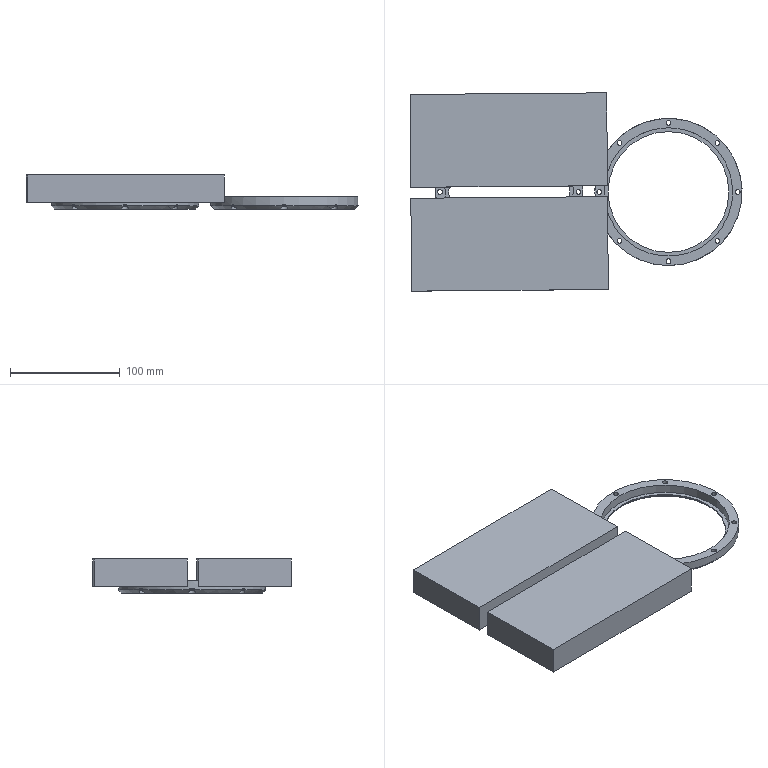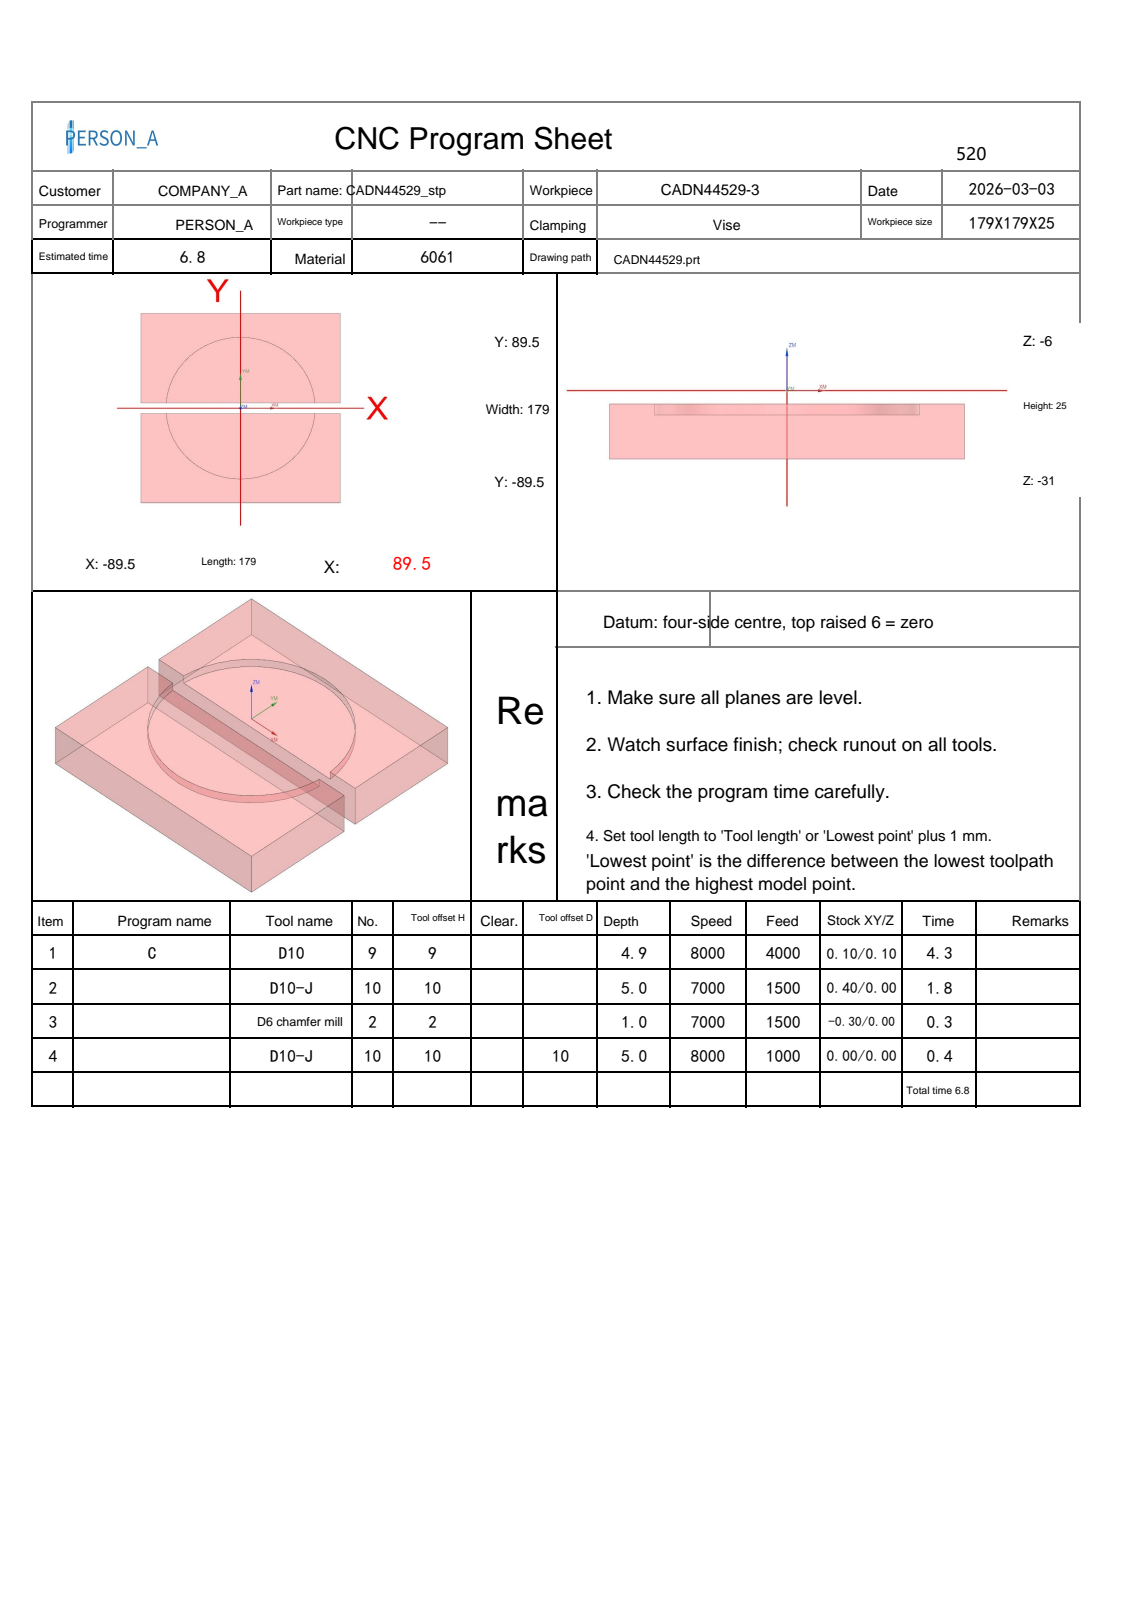NC program | NX | posted by the shop | part box 302.234 x 180.468 x 31 mm
Whole program:
%
O0001
(Machine time: 7.55 MIN)
(===Total Tool:3===)
(T9=D10     D=10.  R=0.   D-  H09 Z=-10.9 )
(T10=D10-J  D=10.  R=0.   D-  H10 Z=-11.  )
(T2=D6 chamfer mill   D=6.   R=0.   D-  H02 Z=-7.   )
G80 G90 G17 G49 G40
G91 G28 Z0
M01
N1 T09 M06
(D10  D=10. R=0. H=09 ce=0.10 di=0.10)
G00 G90 G54 X5.978 Y2.842 M03 S8000
G43 H09 Z4.1
M08
Z-4.5
G03 X5.978 Y2.842 Z-5.982 I-3.383 J-2.967 F4000.
X-1.902 Y.036 Z-6.544 I-3.383 J-2.967
G01 X-1.9 Y-.07
G03 X-.001 Y-1.9 I1.899 J.07
G01 X.142 Y-1.895
G03 X1.895 Y-.142 I-.142 J1.895
G01 X1.9 Y-.07
Y.07
G03 X.001 Y1.9 I-1.899 J-.07
G01 X-.142 Y1.895
X-.304 Y1.876
G03 X-.536 Y1.808 I.16 J-.987
G01 X-8.42 Y-1.553
G03 X-9.028 Y-2.473 I.392 J-.92
X-8.984 Y-2.767 I1. J0.0
X0.0 Y-9.4 I8.984 J2.767
X9.374 Y-.701 I0.0 J9.4
G01 X9.421 Y-.07
Y.07
X9.374 Y.701
G03 X0.0 Y9.4 I-9.374 J-.701
X-8.773 Y3.376 I0.0 J-9.4
G02 X-9.224 Y2.859 I-.933 J.359
G01 X-16.269 Y-1.02
G03 X-16.787 Y-1.896 I.483 J-.876
G01 X-16.779 Y-2.015
G03 X0.0 Y-16.9 I16.779 J2.015
X16.853 Y-1.261 I0.0 J16.9
G01 X16.942 Y-.071
Y.071
X16.853 Y1.261
G03 X0.0 Y16.9 I-16.853 J-1.261
X-16.409 Y4.046 I0.0 J-16.9
G02 X-16.892 Y3.412 I-.971 J.24
G01 X-23.852 Y-.467
G03 X-24.365 Y-1.341 I.487 J-.873
G01 X-24.362 Y-1.415
X-24.332 Y-1.821
G03 X0.0 Y-24.4 I24.332 J1.821
X24.332 Y-1.821 I0.0 J24.4
G01 X24.463 Y-.071
Y.071
X24.332 Y1.821
G03 X0.0 Y24.4 I-24.332 J-1.821
X-23.953 Y4.649 I0.0 J-24.4
G02 X-24.448 Y3.967 I-.982 J.191
G01 X-31.414 Y.092
G03 X-31.928 Y-.782 I.486 J-.874
G01 X-31.925 Y-.856
X-31.811 Y-2.381
G03 X0.0 Y-31.9 I31.811 J2.381
X31.811 Y-2.381 I0.0 J31.9
G01 X31.984 Y-.071
Y.071
X31.811 Y2.381
G03 X0.0 Y31.9 I-31.811 J-2.381
X-31.468 Y5.232 I0.0 J-31.9
G02 X-31.968 Y4.522 I-.986 J.164
G01 X-38.975 Y.625
G03 X-39.489 Y-.249 I.487 J-.874
G01 X-39.486 Y-.323
X-39.29 Y-2.94
G03 X0.0 Y-39.4 I39.29 J2.94
X39.29 Y-2.94 I0.0 J39.4
G01 X39.505 Y-.071
Y.071
X39.29 Y2.94
G03 X0.0 Y39.4 I-39.29 J-2.94
X-38.97 Y5.805 I0.0 J-39.4
G02 X-39.472 Y5.079 I-.989 J.148
G01 X-46.494 Y1.163
G03 X-47.004 Y.365 I.488 J-.873
G01 X-47.026 Y.072
Y-.072
X-46.769 Y-3.5
G03 X0.0 Y-46.9 I46.769 J3.5
X46.769 Y-3.5 I0.0 J46.9
G01 X47.026 Y-.072
Y.072
X46.769 Y3.5
G03 X0.0 Y46.9 I-46.769 J-3.5
X-46.465 Y6.373 I0.0 J-46.9
G02 X-46.967 Y5.637 I-.991 J.136
G01 X-53.974 Y1.723
G03 X-54.483 Y.925 I.488 J-.873
G01 X-54.547 Y.072
Y-.072
X-54.248 Y-4.06
G03 X0.0 Y-54.4 I54.248 J4.06
X54.248 Y-4.06 I0.0 J54.4
G01 X54.547 Y-.072
Y.072
X54.248 Y4.06
G03 X0.0 Y54.4 I-54.248 J-4.06
X-53.923 Y7.188 I0.0 J-54.4
G02 X-54.768 Y6.331 I-.991 J.133
G01 X-60.884 Y5.428
G03 X-61.735 Y4.513 I.146 J-.989
G01 X-62.073 Y0.0
X-61.727 Y-4.619
G03 X0.0 Y-61.9 I61.727 J4.619
X61.727 Y-4.619 I0.0 J61.9
G01 X62.073 Y0.0
X61.727 Y4.619
G03 X0.0 Y61.9 I-61.727 J-4.619
X-61.727 Y4.619 I0.0 J-61.9
G01 X-62.073 Y0.0
X-62.038 Y-.473
X-62. Y-.971
X-59.009 Y-.747
Z-5.044
G00 X5.978 Y2.842
G03 X5.978 Y2.842 Z-6.526 I-3.383 J-2.967
X-1.902 Y.036 Z-7.089 I-3.383 J-2.967
G01 X-1.9 Y-.07
G03 X-.001 Y-1.9 I1.899 J.07
G01 X.142 Y-1.895
G03 X1.895 Y-.142 I-.142 J1.895
G01 X1.9 Y-.07
Y.07
G03 X.001 Y1.9 I-1.899 J-.07
G01 X-.142 Y1.895
X-.304 Y1.876
G03 X-.536 Y1.808 I.16 J-.987
G01 X-8.42 Y-1.553
G03 X-9.028 Y-2.473 I.392 J-.92
X-8.984 Y-2.767 I1. J0.0
X0.0 Y-9.4 I8.984 J2.767
X9.374 Y-.701 I0.0 J9.4
G01 X9.421 Y-.07
Y.07
X9.374 Y.701
G03 X0.0 Y9.4 I-9.374 J-.701
X-8.773 Y3.376 I0.0 J-9.4
G02 X-9.224 Y2.859 I-.933 J.359
G01 X-16.269 Y-1.02
G03 X-16.787 Y-1.896 I.483 J-.876
G01 X-16.779 Y-2.015
G03 X0.0 Y-16.9 I16.779 J2.015
X16.853 Y-1.261 I0.0 J16.9
G01 X16.942 Y-.071
Y.071
X16.853 Y1.261
G03 X0.0 Y16.9 I-16.853 J-1.261
X-16.409 Y4.046 I0.0 J-16.9
G02 X-16.892 Y3.412 I-.971 J.24
G01 X-23.852 Y-.467
G03 X-24.365 Y-1.341 I.487 J-.873
G01 X-24.362 Y-1.415
X-24.332 Y-1.821
G03 X0.0 Y-24.4 I24.332 J1.821
X24.332 Y-1.821 I0.0 J24.4
G01 X24.463 Y-.071
Y.071
X24.332 Y1.821
G03 X0.0 Y24.4 I-24.332 J-1.821
X-23.953 Y4.649 I0.0 J-24.4
G02 X-24.448 Y3.967 I-.982 J.191
G01 X-31.414 Y.092
G03 X-31.928 Y-.782 I.486 J-.874
G01 X-31.925 Y-.856
X-31.811 Y-2.381
G03 X0.0 Y-31.9 I31.811 J2.381
X31.811 Y-2.381 I0.0 J31.9
G01 X31.984 Y-.071
Y.071
X31.811 Y2.381
G03 X0.0 Y31.9 I-31.811 J-2.381
X-31.468 Y5.232 I0.0 J-31.9
G02 X-31.968 Y4.522 I-.986 J.164
G01 X-38.975 Y.625
G03 X-39.489 Y-.249 I.487 J-.874
G01 X-39.486 Y-.323
X-39.29 Y-2.94
G03 X0.0 Y-39.4 I39.29 J2.94
X39.29 Y-2.94 I0.0 J39.4
G01 X39.505 Y-.071
Y.071
X39.29 Y2.94
G03 X0.0 Y39.4 I-39.29 J-2.94
X-38.97 Y5.805 I0.0 J-39.4
G02 X-39.472 Y5.079 I-.989 J.148
G01 X-46.494 Y1.163
G03 X-47.004 Y.365 I.488 J-.873
G01 X-47.026 Y.072
Y-.072
X-46.769 Y-3.5
G03 X0.0 Y-46.9 I46.769 J3.5
X46.769 Y-3.5 I0.0 J46.9
G01 X47.026 Y-.072
Y.072
X46.769 Y3.5
G03 X0.0 Y46.9 I-46.769 J-3.5
X-46.465 Y6.373 I0.0 J-46.9
G02 X-46.967 Y5.637 I-.991 J.136
G01 X-53.974 Y1.723
G03 X-54.483 Y.925 I.488 J-.873
G01 X-54.547 Y.072
Y-.072
X-54.248 Y-4.06
G03 X0.0 Y-54.4 I54.248 J4.06
X54.248 Y-4.06 I0.0 J54.4
G01 X54.547 Y-.072
Y.072
X54.248 Y4.06
G03 X0.0 Y54.4 I-54.248 J-4.06
X-53.923 Y7.188 I0.0 J-54.4
G02 X-54.768 Y6.331 I-.991 J.133
G01 X-60.884 Y5.428
G03 X-61.735 Y4.513 I.146 J-.989
G01 X-62.073 Y0.0
X-61.727 Y-4.619
G03 X0.0 Y-61.9 I61.727 J4.619
X61.727 Y-4.619 I0.0 J61.9
G01 X62.073 Y0.0
X61.727 Y4.619
G03 X0.0 Y61.9 I-61.727 J-4.619
X-61.727 Y4.619 I0.0 J-61.9
G01 X-62.073 Y0.0
X-62.038 Y-.473
X-62. Y-.971
X-59.009 Y-.747
Z-5.589
G00 X5.978 Y2.842
G03 X5.978 Y2.842 Z-7.071 I-3.383 J-2.967
X-1.902 Y.036 Z-7.633 I-3.383 J-2.967
G01 X-1.9 Y-.07
G03 X-.001 Y-1.9 I1.899 J.07
G01 X.142 Y-1.895
G03 X1.895 Y-.142 I-.142 J1.895
G01 X1.9 Y-.07
Y.07
G03 X.001 Y1.9 I-1.899 J-.07
G01 X-.142 Y1.895
X-.304 Y1.876
G03 X-.536 Y1.808 I.16 J-.987
G01 X-8.42 Y-1.553
G03 X-9.028 Y-2.473 I.392 J-.92
X-8.984 Y-2.767 I1. J0.0
X0.0 Y-9.4 I8.984 J2.767
X9.374 Y-.701 I0.0 J9.4
G01 X9.421 Y-.07
Y.07
X9.374 Y.701
G03 X0.0 Y9.4 I-9.374 J-.701
X-8.773 Y3.376 I0.0 J-9.4
G02 X-9.224 Y2.859 I-.933 J.359
G01 X-16.269 Y-1.02
G03 X-16.787 Y-1.896 I.483 J-.876
G01 X-16.779 Y-2.015
G03 X0.0 Y-16.9 I16.779 J2.015
X16.853 Y-1.261 I0.0 J16.9
G01 X16.942 Y-.071
Y.071
X16.853 Y1.261
G03 X0.0 Y16.9 I-16.853 J-1.261
X-16.409 Y4.046 I0.0 J-16.9
G02 X-16.892 Y3.412 I-.971 J.24
G01 X-23.852 Y-.467
G03 X-24.365 Y-1.341 I.487 J-.873
G01 X-24.362 Y-1.415
X-24.332 Y-1.821
G03 X0.0 Y-24.4 I24.332 J1.821
X24.332 Y-1.821 I0.0 J24.4
G01 X24.463 Y-.071
Y.071
X24.332 Y1.821
G03 X0.0 Y24.4 I-24.332 J-1.821
X-23.953 Y4.649 I0.0 J-24.4
G02 X-24.448 Y3.967 I-.982 J.191
G01 X-31.414 Y.092
G03 X-31.928 Y-.782 I.486 J-.874
G01 X-31.925 Y-.856
X-31.811 Y-2.381
G03 X0.0 Y-31.9 I31.811 J2.381
X31.811 Y-2.381 I0.0 J31.9
G01 X31.984 Y-.071
Y.071
X31.811 Y2.381
G03 X0.0 Y31.9 I-31.811 J-2.381
X-31.468 Y5.232 I0.0 J-31.9
G02 X-31.968 Y4.522 I-.986 J.164
G01 X-38.975 Y.625
G03 X-39.489 Y-.249 I.487 J-.874
G01 X-39.486 Y-.323
X-39.29 Y-2.94
G03 X0.0 Y-39.4 I39.29 J2.94
X39.29 Y-2.94 I0.0 J39.4
G01 X39.505 Y-.071
Y.071
X39.29 Y2.94
G03 X0.0 Y39.4 I-39.29 J-2.94
X-38.97 Y5.805 I0.0 J-39.4
G02 X-39.472 Y5.079 I-.989 J.148
G01 X-46.494 Y1.163
G03 X-47.004 Y.365 I.488 J-.873
G01 X-47.026 Y.072
Y-.072
X-46.769 Y-3.5
G03 X0.0 Y-46.9 I46.769 J3.5
X46.769 Y-3.5 I0.0 J46.9
G01 X47.026 Y-.072
Y.072
X46.769 Y3.5
G03 X0.0 Y46.9 I-46.769 J-3.5
X-46.465 Y6.373 I0.0 J-46.9
G02 X-46.967 Y5.637 I-.991 J.136
G01 X-53.974 Y1.723
G03 X-54.483 Y.925 I.488 J-.873
G01 X-54.547 Y.072
Y-.072
X-54.248 Y-4.06
G03 X0.0 Y-54.4 I54.248 J4.06
X54.248 Y-4.06 I0.0 J54.4
G01 X54.547 Y-.072
Y.072
X54.248 Y4.06
G03 X0.0 Y54.4 I-54.248 J-4.06
X-53.923 Y7.188 I0.0 J-54.4
G02 X-54.768 Y6.331 I-.991 J.133
G01 X-60.884 Y5.428
G03 X-61.735 Y4.513 I.146 J-.989
G01 X-62.073 Y0.0
X-61.727 Y-4.619
G03 X0.0 Y-61.9 I61.727 J4.619
X61.727 Y-4.619 I0.0 J61.9
G01 X62.073 Y0.0
X61.727 Y4.619
G03 X0.0 Y61.9 I-61.727 J-4.619
X-61.727 Y4.619 I0.0 J-61.9
G01 X-62.073 Y0.0
X-62.038 Y-.473
X-62. Y-.971
X-59.009 Y-.747
Z-6.133
G00 X5.978 Y2.842
G03 X5.978 Y2.842 Z-7.615 I-3.383 J-2.967
X-1.902 Y.036 Z-8.178 I-3.383 J-2.967
G01 X-1.9 Y-.07
G03 X-.001 Y-1.9 I1.899 J.07
G01 X.142 Y-1.895
G03 X1.895 Y-.142 I-.142 J1.895
G01 X1.9 Y-.07
Y.07
G03 X.001 Y1.9 I-1.899 J-.07
G01 X-.142 Y1.895
X-.304 Y1.876
G03 X-.536 Y1.808 I.16 J-.987
G01 X-8.42 Y-1.553
G03 X-9.028 Y-2.473 I.392 J-.92
X-8.984 Y-2.767 I1. J0.0
X0.0 Y-9.4 I8.984 J2.767
X9.374 Y-.701 I0.0 J9.4
G01 X9.421 Y-.07
Y.07
X9.374 Y.701
G03 X0.0 Y9.4 I-9.374 J-.701
X-8.773 Y3.376 I0.0 J-9.4
G02 X-9.224 Y2.859 I-.933 J.359
G01 X-16.269 Y-1.02
G03 X-16.787 Y-1.896 I.483 J-.876
G01 X-16.779 Y-2.015
G03 X0.0 Y-16.9 I16.779 J2.015
X16.853 Y-1.261 I0.0 J16.9
G01 X16.942 Y-.071
Y.071
X16.853 Y1.261
G03 X0.0 Y16.9 I-16.853 J-1.261
X-16.409 Y4.046 I0.0 J-16.9
G02 X-16.892 Y3.412 I-.971 J.24
G01 X-23.852 Y-.467
G03 X-24.365 Y-1.341 I.487 J-.873
G01 X-24.362 Y-1.415
X-24.332 Y-1.821
G03 X0.0 Y-24.4 I24.332 J1.821
X24.332 Y-1.821 I0.0 J24.4
G01 X24.463 Y-.071
Y.071
X24.332 Y1.821
G03 X0.0 Y24.4 I-24.332 J-1.821
X-23.953 Y4.649 I0.0 J-24.4
G02 X-24.448 Y3.967 I-.982 J.191
G01 X-31.414 Y.092
G03 X-31.928 Y-.782 I.486 J-.874
G01 X-31.925 Y-.856
X-31.811 Y-2.381
G03 X0.0 Y-31.9 I31.811 J2.381
X31.811 Y-2.381 I0.0 J31.9
G01 X31.984 Y-.071
Y.071
X31.811 Y2.381
G03 X0.0 Y31.9 I-31.811 J-2.381
X-31.468 Y5.232 I0.0 J-31.9
G02 X-31.968 Y4.522 I-.986 J.164
G01 X-38.975 Y.625
G03 X-39.489 Y-.249 I.487 J-.874
G01 X-39.486 Y-.323
X-39.29 Y-2.94
G03 X0.0 Y-39.4 I39.29 J2.94
X39.29 Y-2.94 I0.0 J39.4
G01 X39.505 Y-.071
Y.071
X39.29 Y2.94
G03 X0.0 Y39.4 I-39.29 J-2.94
X-38.97 Y5.805 I0.0 J-39.4
G02 X-39.472 Y5.079 I-.989 J.148
G01 X-46.494 Y1.163
G03 X-47.004 Y.365 I.488 J-.873
G01 X-47.026 Y.072
Y-.072
X-46.769 Y-3.5
G03 X0.0 Y-46.9 I46.769 J3.5
X46.769 Y-3.5 I0.0 J46.9
G01 X47.026 Y-.072
Y.072
X46.769 Y3.5
G03 X0.0 Y46.9 I-46.769 J-3.5
X-46.465 Y6.373 I0.0 J-46.9
G02 X-46.967 Y5.637 I-.991 J.136
G01 X-53.974 Y1.723
G03 X-54.483 Y.925 I.488 J-.873
G01 X-54.547 Y.072
Y-.072
X-54.248 Y-4.06
G03 X0.0 Y-54.4 I54.248 J4.06
X54.248 Y-4.06 I0.0 J54.4
G01 X54.547 Y-.072
Y.072
X54.248 Y4.06
G03 X0.0 Y54.4 I-54.248 J-4.06
X-53.923 Y7.188 I0.0 J-54.4
G02 X-54.768 Y6.331 I-.991 J.133
G01 X-60.884 Y5.428
G03 X-61.735 Y4.513 I.146 J-.989
G01 X-62.073 Y0.0
X-61.727 Y-4.619
G03 X0.0 Y-61.9 I61.727 J4.619
X61.727 Y-4.619 I0.0 J61.9
G01 X62.073 Y0.0
X61.727 Y4.619
G03 X0.0 Y61.9 I-61.727 J-4.619
X-61.727 Y4.619 I0.0 J-61.9
G01 X-62.073 Y0.0
X-62.038 Y-.473
X-62. Y-.971
X-59.009 Y-.747
Z-6.678
G00 X5.978 Y2.842
G03 X5.978 Y2.842 Z-8.16 I-3.383 J-2.967
X-1.902 Y.036 Z-8.722 I-3.383 J-2.967
G01 X-1.9 Y-.07
G03 X-.001 Y-1.9 I1.899 J.07
G01 X.142 Y-1.895
G03 X1.895 Y-.142 I-.142 J1.895
G01 X1.9 Y-.07
Y.07
G03 X.001 Y1.9 I-1.899 J-.07
G01 X-.142 Y1.895
X-.304 Y1.876
G03 X-.536 Y1.808 I.16 J-.987
G01 X-8.42 Y-1.553
G03 X-9.028 Y-2.473 I.392 J-.92
X-8.984 Y-2.767 I1. J0.0
X0.0 Y-9.4 I8.984 J2.767
X9.374 Y-.701 I0.0 J9.4
G01 X9.421 Y-.07
Y.07
X9.374 Y.701
G03 X0.0 Y9.4 I-9.374 J-.701
X-8.773 Y3.376 I0.0 J-9.4
G02 X-9.224 Y2.859 I-.933 J.359
G01 X-16.269 Y-1.02
G03 X-16.787 Y-1.896 I.483 J-.876
G01 X-16.779 Y-2.015
G03 X0.0 Y-16.9 I16.779 J2.015
X16.853 Y-1.261 I0.0 J16.9
G01 X16.942 Y-.071
Y.071
X16.853 Y1.261
G03 X0.0 Y16.9 I-16.853 J-1.261
X-16.409 Y4.046 I0.0 J-16.9
G02 X-16.892 Y3.412 I-.971 J.24
G01 X-23.852 Y-.467
G03 X-24.365 Y-1.341 I.487 J-.873
G01 X-24.362 Y-1.415
X-24.332 Y-1.821
G03 X0.0 Y-24.4 I24.332 J1.821
X24.332 Y-1.821 I0.0 J24.4
G01 X24.463 Y-.071
Y.071
X24.332 Y1.821
G03 X0.0 Y24.4 I-24.332 J-1.821
X-23.953 Y4.649 I0.0 J-24.4
G02 X-24.448 Y3.967 I-.982 J.191
G01 X-31.414 Y.092
G03 X-31.928 Y-.782 I.486 J-.874
G01 X-31.925 Y-.856
X-31.811 Y-2.381
G03 X0.0 Y-31.9 I31.811 J2.381
X31.811 Y-2.381 I0.0 J31.9
G01 X31.984 Y-.071
Y.071
X31.811 Y2.381
G03 X0.0 Y31.9 I-31.811 J-2.381
X-31.468 Y5.232 I0.0 J-31.9
G02 X-31.968 Y4.522 I-.986 J.164
G01 X-38.975 Y.625
G03 X-39.489 Y-.249 I.487 J-.874
G01 X-39.486 Y-.323
X-39.29 Y-2.94
G03 X0.0 Y-39.4 I39.29 J2.94
X39.29 Y-2.94 I0.0 J39.4
G01 X39.505 Y-.071
Y.071
X39.29 Y2.94
G03 X0.0 Y39.4 I-39.29 J-2.94
X-38.97 Y5.805 I0.0 J-39.4
G02 X-39.472 Y5.079 I-.989 J.148
G01 X-46.494 Y1.163
G03 X-47.004 Y.365 I.488 J-.873
G01 X-47.026 Y.072
Y-.072
X-46.769 Y-3.5
G03 X0.0 Y-46.9 I46.769 J3.5
X46.769 Y-3.5 I0.0 J46.9
G01 X47.026 Y-.072
Y.072
X46.769 Y3.5
G03 X0.0 Y46.9 I-46.769 J-3.5
X-46.465 Y6.373 I0.0 J-46.9
G02 X-46.967 Y5.637 I-.991 J.136
G01 X-53.974 Y1.723
G03 X-54.483 Y.925 I.488 J-.873
G01 X-54.547 Y.072
Y-.072
X-54.248 Y-4.06
G03 X0.0 Y-54.4 I54.248 J4.06
X54.248 Y-4.06 I0.0 J54.4
G01 X54.547 Y-.072
Y.072
X54.248 Y4.06
G03 X0.0 Y54.4 I-54.248 J-4.06
X-53.923 Y7.188 I0.0 J-54.4
G02 X-54.768 Y6.331 I-.991 J.133
G01 X-60.884 Y5.428
G03 X-61.735 Y4.513 I.146 J-.989
G01 X-62.073 Y0.0
X-61.727 Y-4.619
G03 X0.0 Y-61.9 I61.727 J4.619
X61.727 Y-4.619 I0.0 J61.9
G01 X62.073 Y0.0
X61.727 Y4.619
G03 X0.0 Y61.9 I-61.727 J-4.619
X-61.727 Y4.619 I0.0 J-61.9
G01 X-62.073 Y0.0
X-62.038 Y-.473
X-62. Y-.971
X-59.009 Y-.747
Z-7.222
G00 X5.978 Y2.842
G03 X5.978 Y2.842 Z-8.704 I-3.383 J-2.967
X-1.902 Y.036 Z-9.267 I-3.383 J-2.967
G01 X-1.9 Y-.07
G03 X-.001 Y-1.9 I1.899 J.07
G01 X.142 Y-1.895
G03 X1.895 Y-.142 I-.142 J1.895
G01 X1.9 Y-.07
Y.07
G03 X.001 Y1.9 I-1.899 J-.07
G01 X-.142 Y1.895
X-.304 Y1.876
G03 X-.536 Y1.808 I.16 J-.987
G01 X-8.42 Y-1.553
G03 X-9.028 Y-2.473 I.392 J-.92
X-8.984 Y-2.767 I1. J0.0
X0.0 Y-9.4 I8.984 J2.767
X9.374 Y-.701 I0.0 J9.4
G01 X9.421 Y-.07
Y.07
X9.374 Y.701
G03 X0.0 Y9.4 I-9.374 J-.701
X-8.773 Y3.376 I0.0 J-9.4
G02 X-9.224 Y2.859 I-.933 J.359
G01 X-16.269 Y-1.02
G03 X-16.787 Y-1.896 I.483 J-.876
G01 X-16.779 Y-2.015
G03 X0.0 Y-16.9 I16.779 J2.015
X16.853 Y-1.261 I0.0 J16.9
G01 X16.942 Y-.071
Y.071
X16.853 Y1.261
G03 X0.0 Y16.9 I-16.853 J-1.261
X-16.409 Y4.046 I0.0 J-16.9
G02 X-16.892 Y3.412 I-.971 J.24
G01 X-23.852 Y-.467
G03 X-24.365 Y-1.341 I.487 J-.873
G01 X-24.362 Y-1.415
X-24.332 Y-1.821
G03 X0.0 Y-24.4 I24.332 J1.821
X24.332 Y-1.821 I0.0 J24.4
G01 X24.463 Y-.071
Y.071
X24.332 Y1.821
G03 X0.0 Y24.4 I-24.332 J-1.821
X-23.953 Y4.649 I0.0 J-24.4
G02 X-24.448 Y3.967 I-.982 J.191
G01 X-31.414 Y.092
G03 X-31.928 Y-.782 I.486 J-.874
G01 X-31.925 Y-.856
X-31.811 Y-2.381
G03 X0.0 Y-31.9 I31.811 J2.381
X31.811 Y-2.381 I0.0 J31.9
G01 X31.984 Y-.071
Y.071
X31.811 Y2.381
G03 X0.0 Y31.9 I-31.811 J-2.381
X-31.468 Y5.232 I0.0 J-31.9
G02 X-31.968 Y4.522 I-.986 J.164
G01 X-38.975 Y.625
G03 X-39.489 Y-.249 I.487 J-.874
G01 X-39.486 Y-.323
X-39.29 Y-2.94
G03 X0.0 Y-39.4 I39.29 J2.94
X39.29 Y-2.94 I0.0 J39.4
G01 X39.505 Y-.071
Y.071
X39.29 Y2.94
G03 X0.0 Y39.4 I-39.29 J-2.94
X-38.97 Y5.805 I0.0 J-39.4
G02 X-39.472 Y5.079 I-.989 J.148
G01 X-46.494 Y1.163
G03 X-47.004 Y.365 I.488 J-.873
G01 X-47.026 Y.072
Y-.072
X-46.769 Y-3.5
G03 X0.0 Y-46.9 I46.769 J3.5
X46.769 Y-3.5 I0.0 J46.9
G01 X47.026 Y-.072
Y.072
X46.769 Y3.5
G03 X0.0 Y46.9 I-46.769 J-3.5
X-46.465 Y6.373 I0.0 J-46.9
G02 X-46.967 Y5.637 I-.991 J.136
G01 X-53.974 Y1.723
G03 X-54.483 Y.925 I.488 J-.873
G01 X-54.547 Y.072
Y-.072
X-54.248 Y-4.06
G03 X0.0 Y-54.4 I54.248 J4.06
X54.248 Y-4.06 I0.0 J54.4
G01 X54.547 Y-.072
Y.072
X54.248 Y4.06
G03 X0.0 Y54.4 I-54.248 J-4.06
X-53.923 Y7.188 I0.0 J-54.4
G02 X-54.768 Y6.331 I-.991 J.133
G01 X-60.884 Y5.428
G03 X-61.735 Y4.513 I.146 J-.989
G01 X-62.073 Y0.0
X-61.727 Y-4.619
G03 X0.0 Y-61.9 I61.727 J4.619
X61.727 Y-4.619 I0.0 J61.9
G01 X62.073 Y0.0
X61.727 Y4.619
G03 X0.0 Y61.9 I-61.727 J-4.619
X-61.727 Y4.619 I0.0 J-61.9
G01 X-62.073 Y0.0
X-62.038 Y-.473
X-62. Y-.971
X-59.009 Y-.747
Z-7.767
G00 X5.978 Y2.842
G03 X5.978 Y2.842 Z-9.249 I-3.383 J-2.967
X-1.902 Y.036 Z-9.811 I-3.383 J-2.967
G01 X-1.9 Y-.07
G03 X-.001 Y-1.9 I1.899 J.07
G01 X.142 Y-1.895
G03 X1.895 Y-.142 I-.142 J1.895
G01 X1.9 Y-.07
Y.07
G03 X.001 Y1.9 I-1.899 J-.07
G01 X-.142 Y1.895
X-.304 Y1.876
G03 X-.536 Y1.808 I.16 J-.987
G01 X-8.42 Y-1.553
G03 X-9.028 Y-2.473 I.392 J-.92
X-8.984 Y-2.767 I1. J0.0
X0.0 Y-9.4 I8.984 J2.767
X9.374 Y-.701 I0.0 J9.4
G01 X9.421 Y-.07
Y.07
X9.374 Y.701
G03 X0.0 Y9.4 I-9.374 J-.701
X-8.773 Y3.376 I0.0 J-9.4
G02 X-9.224 Y2.859 I-.933 J.359
G01 X-16.269 Y-1.02
G03 X-16.787 Y-1.896 I.483 J-.876
G01 X-16.779 Y-2.015
G03 X0.0 Y-16.9 I16.779 J2.015
X16.853 Y-1.261 I0.0 J16.9
G01 X16.942 Y-.071
Y.071
X16.853 Y1.261
G03 X0.0 Y16.9 I-16.853 J-1.261
X-16.409 Y4.046 I0.0 J-16.9
G02 X-16.892 Y3.412 I-.971 J.24
G01 X-23.852 Y-.467
G03 X-24.365 Y-1.341 I.487 J-.873
G01 X-24.362 Y-1.415
X-24.332 Y-1.821
G03 X0.0 Y-24.4 I24.332 J1.821
X24.332 Y-1.821 I0.0 J24.4
G01 X24.463 Y-.071
Y.071
X24.332 Y1.821
G03 X0.0 Y24.4 I-24.332 J-1.821
X-23.953 Y4.649 I0.0 J-24.4
G02 X-24.448 Y3.967 I-.982 J.191
G01 X-31.414 Y.092
G03 X-31.928 Y-.782 I.486 J-.874
G01 X-31.925 Y-.856
X-31.811 Y-2.381
G03 X0.0 Y-31.9 I31.811 J2.381
X31.811 Y-2.381 I0.0 J31.9
G01 X31.984 Y-.071
Y.071
X31.811 Y2.381
G03 X0.0 Y31.9 I-31.811 J-2.381
X-31.468 Y5.232 I0.0 J-31.9
G02 X-31.968 Y4.522 I-.986 J.164
G01 X-38.975 Y.625
G03 X-39.489 Y-.249 I.487 J-.874
G01 X-39.486 Y-.323
X-39.29 Y-2.94
G03 X0.0 Y-39.4 I39.29 J2.94
X39.29 Y-2.94 I0.0 J39.4
G01 X39.505 Y-.071
Y.071
X39.29 Y2.94
G03 X0.0 Y39.4 I-39.29 J-2.94
X-38.97 Y5.805 I0.0 J-39.4
G02 X-39.472 Y5.079 I-.989 J.148
G01 X-46.494 Y1.163
G03 X-47.004 Y.365 I.488 J-.873
G01 X-47.026 Y.072
Y-.072
X-46.769 Y-3.5
G03 X0.0 Y-46.9 I46.769 J3.5
X46.769 Y-3.5 I0.0 J46.9
G01 X47.026 Y-.072
Y.072
X46.769 Y3.5
G03 X0.0 Y46.9 I-46.769 J-3.5
X-46.465 Y6.373 I0.0 J-46.9
G02 X-46.967 Y5.637 I-.991 J.136
G01 X-53.974 Y1.723
G03 X-54.483 Y.925 I.488 J-.873
G01 X-54.547 Y.072
Y-.072
X-54.248 Y-4.06
G03 X0.0 Y-54.4 I54.248 J4.06
X54.248 Y-4.06 I0.0 J54.4
G01 X54.547 Y-.072
Y.072
X54.248 Y4.06
G03 X0.0 Y54.4 I-54.248 J-4.06
X-53.923 Y7.188 I0.0 J-54.4
G02 X-54.768 Y6.331 I-.991 J.133
G01 X-60.884 Y5.428
G03 X-61.735 Y4.513 I.146 J-.989
G01 X-62.073 Y0.0
X-61.727 Y-4.619
G03 X0.0 Y-61.9 I61.727 J4.619
X61.727 Y-4.619 I0.0 J61.9
G01 X62.073 Y0.0
X61.727 Y4.619
G03 X0.0 Y61.9 I-61.727 J-4.619
X-61.727 Y4.619 I0.0 J-61.9
G01 X-62.073 Y0.0
X-62.038 Y-.473
X-62. Y-.971
X-59.009 Y-.747
Z-8.311
G00 X5.978 Y2.842
G03 X5.978 Y2.842 Z-9.793 I-3.383 J-2.967
X-1.902 Y.036 Z-10.356 I-3.383 J-2.967
G01 X-1.9 Y-.07
G03 X-.001 Y-1.9 I1.899 J.07
G01 X.142 Y-1.895
G03 X1.895 Y-.142 I-.142 J1.895
G01 X1.9 Y-.07
Y.07
G03 X.001 Y1.9 I-1.899 J-.07
G01 X-.142 Y1.895
X-.304 Y1.876
G03 X-.536 Y1.808 I.16 J-.987
G01 X-8.42 Y-1.553
G03 X-9.028 Y-2.473 I.392 J-.92
X-8.984 Y-2.767 I1. J0.0
X0.0 Y-9.4 I8.984 J2.767
X9.374 Y-.701 I0.0 J9.4
G01 X9.421 Y-.07
Y.07
X9.374 Y.701
G03 X0.0 Y9.4 I-9.374 J-.701
X-8.773 Y3.376 I0.0 J-9.4
G02 X-9.224 Y2.859 I-.933 J.359
G01 X-16.269 Y-1.02
G03 X-16.787 Y-1.896 I.483 J-.876
G01 X-16.779 Y-2.015
G03 X0.0 Y-16.9 I16.779 J2.015
X16.853 Y-1.261 I0.0 J16.9
G01 X16.942 Y-.071
Y.071
X16.853 Y1.261
G03 X0.0 Y16.9 I-16.853 J-1.261
X-16.409 Y4.046 I0.0 J-16.9
G02 X-16.892 Y3.412 I-.971 J.24
G01 X-23.852 Y-.467
G03 X-24.365 Y-1.341 I.487 J-.873
G01 X-24.362 Y-1.415
X-24.332 Y-1.821
G03 X0.0 Y-24.4 I24.332 J1.821
X24.332 Y-1.821 I0.0 J24.4
G01 X24.463 Y-.071
Y.071
X24.332 Y1.821
G03 X0.0 Y24.4 I-24.332 J-1.821
X-23.953 Y4.649 I0.0 J-24.4
G02 X-24.448 Y3.967 I-.982 J.191
G01 X-31.414 Y.092
G03 X-31.928 Y-.782 I.486 J-.874
G01 X-31.925 Y-.856
X-31.811 Y-2.381
G03 X0.0 Y-31.9 I31.811 J2.381
X31.811 Y-2.381 I0.0 J31.9
G01 X31.984 Y-.071
Y.071
X31.811 Y2.381
G03 X0.0 Y31.9 I-31.811 J-2.381
X-31.468 Y5.232 I0.0 J-31.9
G02 X-31.968 Y4.522 I-.986 J.164
G01 X-38.975 Y.625
G03 X-39.489 Y-.249 I.487 J-.874
G01 X-39.486 Y-.323
X-39.29 Y-2.94
G03 X0.0 Y-39.4 I39.29 J2.94
X39.29 Y-2.94 I0.0 J39.4
G01 X39.505 Y-.071
Y.071
X39.29 Y2.94
G03 X0.0 Y39.4 I-39.29 J-2.94
X-38.97 Y5.805 I0.0 J-39.4
G02 X-39.472 Y5.079 I-.989 J.148
G01 X-46.494 Y1.163
G03 X-47.004 Y.365 I.488 J-.873
G01 X-47.026 Y.072
Y-.072
X-46.769 Y-3.5
G03 X0.0 Y-46.9 I46.769 J3.5
X46.769 Y-3.5 I0.0 J46.9
G01 X47.026 Y-.072
Y.072
X46.769 Y3.5
G03 X0.0 Y46.9 I-46.769 J-3.5
X-46.465 Y6.373 I0.0 J-46.9
G02 X-46.967 Y5.637 I-.991 J.136
G01 X-53.974 Y1.723
G03 X-54.483 Y.925 I.488 J-.873
G01 X-54.547 Y.072
Y-.072
X-54.248 Y-4.06
G03 X0.0 Y-54.4 I54.248 J4.06
X54.248 Y-4.06 I0.0 J54.4
G01 X54.547 Y-.072
Y.072
X54.248 Y4.06
G03 X0.0 Y54.4 I-54.248 J-4.06
X-53.923 Y7.188 I0.0 J-54.4
G02 X-54.768 Y6.331 I-.991 J.133
G01 X-60.884 Y5.428
G03 X-61.735 Y4.513 I.146 J-.989
G01 X-62.073 Y0.0
X-61.727 Y-4.619
G03 X0.0 Y-61.9 I61.727 J4.619
X61.727 Y-4.619 I0.0 J61.9
G01 X62.073 Y0.0
X61.727 Y4.619
G03 X0.0 Y61.9 I-61.727 J-4.619
X-61.727 Y4.619 I0.0 J-61.9
G01 X-62.073 Y0.0
X-62.038 Y-.473
X-62. Y-.971
X-59.009 Y-.747
Z-8.856
G00 X5.978 Y2.842
G03 X5.978 Y2.842 Z-10.337 I-3.383 J-2.967
X-1.902 Y.036 Z-10.9 I-3.383 J-2.967
G01 X-1.9 Y-.07
G03 X-.001 Y-1.9 I1.899 J.07
G01 X.142 Y-1.895
G03 X1.895 Y-.142 I-.142 J1.895
G01 X1.9 Y-.07
Y.07
G03 X.001 Y1.9 I-1.899 J-.07
G01 X-.142 Y1.895
X-.304 Y1.876
G03 X-.536 Y1.808 I.16 J-.987
G01 X-8.42 Y-1.553
G03 X-9.028 Y-2.473 I.392 J-.92
X-8.984 Y-2.767 I1. J0.0
X0.0 Y-9.4 I8.984 J2.767
X9.374 Y-.701 I0.0 J9.4
G01 X9.421 Y-.07
Y.07
X9.374 Y.701
G03 X0.0 Y9.4 I-9.374 J-.701
X-8.773 Y3.376 I0.0 J-9.4
G02 X-9.224 Y2.859 I-.933 J.359
G01 X-16.269 Y-1.02
G03 X-16.787 Y-1.896 I.483 J-.876
G01 X-16.779 Y-2.015
G03 X0.0 Y-16.9 I16.779 J2.015
X16.853 Y-1.261 I0.0 J16.9
G01 X16.942 Y-.071
Y.071
X16.853 Y1.261
G03 X0.0 Y16.9 I-16.853 J-1.261
X-16.409 Y4.046 I0.0 J-16.9
G02 X-16.892 Y3.412 I-.971 J.24
G01 X-23.852 Y-.467
G03 X-24.365 Y-1.341 I.487 J-.873
G01 X-24.362 Y-1.415
X-24.332 Y-1.821
G03 X0.0 Y-24.4 I24.332 J1.821
X24.332 Y-1.821 I0.0 J24.4
G01 X24.463 Y-.071
Y.071
X24.332 Y1.821
G03 X0.0 Y24.4 I-24.332 J-1.821
X-23.953 Y4.649 I0.0 J-24.4
G02 X-24.448 Y3.967 I-.982 J.191
G01 X-31.414 Y.092
G03 X-31.928 Y-.782 I.486 J-.874
G01 X-31.925 Y-.856
X-31.811 Y-2.381
G03 X0.0 Y-31.9 I31.811 J2.381
X31.811 Y-2.381 I0.0 J31.9
G01 X31.984 Y-.071
Y.071
X31.811 Y2.381
G03 X0.0 Y31.9 I-31.811 J-2.381
X-31.468 Y5.232 I0.0 J-31.9
G02 X-31.968 Y4.522 I-.986 J.164
G01 X-38.975 Y.625
G03 X-39.489 Y-.249 I.487 J-.874
G01 X-39.486 Y-.323
X-39.29 Y-2.94
G03 X0.0 Y-39.4 I39.29 J2.94
X39.29 Y-2.94 I0.0 J39.4
G01 X39.505 Y-.071
Y.071
X39.29 Y2.94
G03 X0.0 Y39.4 I-39.29 J-2.94
X-38.97 Y5.805 I0.0 J-39.4
G02 X-39.472 Y5.079 I-.989 J.148
G01 X-46.494 Y1.163
G03 X-47.004 Y.365 I.488 J-.873
G01 X-47.026 Y.072
Y-.072
X-46.769 Y-3.5
G03 X0.0 Y-46.9 I46.769 J3.5
X46.769 Y-3.5 I0.0 J46.9
G01 X47.026 Y-.072
Y.072
X46.769 Y3.5
G03 X0.0 Y46.9 I-46.769 J-3.5
X-46.465 Y6.373 I0.0 J-46.9
G02 X-46.967 Y5.637 I-.991 J.136
G01 X-53.974 Y1.723
G03 X-54.483 Y.925 I.488 J-.873
G01 X-54.547 Y.072
Y-.072
X-54.248 Y-4.06
G03 X0.0 Y-54.4 I54.248 J4.06
X54.248 Y-4.06 I0.0 J54.4
G01 X54.547 Y-.072
Y.072
X54.248 Y4.06
G03 X0.0 Y54.4 I-54.248 J-4.06
X-53.923 Y7.188 I0.0 J-54.4
G02 X-54.768 Y6.331 I-.991 J.133
G01 X-60.884 Y5.428
G03 X-61.735 Y4.513 I.146 J-.989
G01 X-62.073 Y0.0
X-61.727 Y-4.619
G03 X0.0 Y-61.9 I61.727 J4.619
X61.727 Y-4.619 I0.0 J61.9
G01 X62.073 Y0.0
X61.727 Y4.619
G03 X0.0 Y61.9 I-61.727 J-4.619
X-61.727 Y4.619 I0.0 J-61.9
G01 X-62.073 Y0.0
X-62.038 Y-.473
X-62. Y-.971
X-59.009 Y-.747
Z-9.4
G00 Z4.1
G91 G28 Z0.0
M05
M09
G91 G28 Z0.0
M01
N2 T10 M06
(D10-J  D=10. R=0. H=10 ce=0.40 di=0.00)
G00 G90 G54 X55.419 Y11.516 M03 S7000
G43 H10 Z4.4
M08
Z-9.
G01 X55.49 Y11.204 Z-9.086 F1500.
X56.005 Y8.256 Z-9.888
X56.363 Y5.285 Z-10.69
X56.449 Y4.13 Z-11.
X61.435 Y4.503
X61.767 Y.072
X61.779 Y0.0
X61.767 Y-.072
X61.428 Y-4.597
G02 X0.0 Y-61.6 I-61.428 J4.597
X-61.428 Y-4.597 I0.0 J61.6
G01 X-61.767 Y-.072
X-61.779 Y0.0
X-61.767 Y.072
X-61.428 Y4.597
G02 X0.0 Y61.6 I61.428 J-4.597
X61.428 Y4.597 I0.0 J-61.6
G01 X61.767 Y.072
X61.779 Y0.0
X61.767 Y-.072
X61.736 Y-.484
G02 X61.006 Y-1.373 I-.997 J.075
G01 X57.241 Y-2.416
G03 X56.511 Y-3.304 I.268 J-.964
G01 X56.442 Y-4.224
G02 X0.0 Y-56.6 I-56.442 J4.224
X-56.442 Y-4.224 I0.0 J56.6
G01 X-56.753 Y-.072
X-56.765 Y0.0
X-56.753 Y.072
X-56.442 Y4.224
G02 X0.0 Y56.6 I56.442 J-4.224
X56.442 Y4.224 I0.0 J-56.6
G01 X56.545 Y2.848
X56.548 Y2.774
G02 X56.246 Y2.057 I-1. J0.0
G01 X51.827 Y-2.248
G03 X51.528 Y-2.888 I.698 J-.716
G01 X51.456 Y-3.851
G02 X0.0 Y-51.6 I-51.456 J3.851
X-51.456 Y-3.851 I0.0 J51.6
G01 X-51.739 Y-.071
X-51.751 Y0.0
X-51.739 Y.071
X-51.456 Y3.851
G02 X0.0 Y51.6 I51.456 J-3.851
X51.456 Y3.851 I0.0 J-51.6
G01 X51.525 Y2.935
X51.527 Y2.86
G02 X51.232 Y2.15 I-1. J0.0
G01 X46.809 Y-2.234
G03 X46.516 Y-2.868 I.704 J-.71
G01 X46.47 Y-3.478
G02 X0.0 Y-46.6 I-46.47 J3.478
X-46.47 Y-3.478 I0.0 J46.6
G01 X-46.725 Y-.071
X-46.738 Y0.0
X-46.725 Y.071
X-46.47 Y3.478
G02 X0.0 Y46.6 I46.47 J-3.478
X46.47 Y3.478 I0.0 J-46.6
G01 X46.51 Y2.949
X46.512 Y2.875
G02 X46.218 Y2.166 I-1. J0.0
G01 X41.794 Y-2.231
G03 X41.502 Y-2.865 I.705 J-.709
G01 X41.484 Y-3.104
G02 X0.0 Y-41.6 I-41.484 J3.104
X-41.484 Y-3.104 I0.0 J41.6
G01 X-41.711 Y-.071
X-41.724 Y0.0
X-41.711 Y.071
X-41.484 Y3.104
G02 X0.0 Y41.6 I41.484 J-3.104
X41.484 Y3.104 I0.0 J-41.6
G01 X41.495 Y2.951
X41.498 Y2.877
G02 X41.204 Y2.168 I-1. J0.0
G01 X36.779 Y-2.231
G03 X36.488 Y-2.861 I.705 J-.709
G02 X0.0 Y-36.6 I-36.488 J2.861
X-36.498 Y-2.731 I0.0 J36.6
G01 X-36.697 Y-.07
Y.07
X-36.498 Y2.731
G02 X0.0 Y36.6 I36.498 J-2.731
X36.48 Y2.957 I0.0 J-36.6
G01 X36.484 Y2.877
G02 X36.189 Y2.168 I-1. J0.0
G01 X31.761 Y-2.235
G03 X31.471 Y-2.853 I.705 J-.709
G02 X0.0 Y-31.6 I-31.471 J2.853
X-31.512 Y-2.358 I0.0 J31.6
G01 X-31.683 Y-.07
Y.07
X-31.512 Y2.358
G02 X0.0 Y31.6 I31.512 J-2.358
X31.46 Y2.966 I0.0 J-31.6
G01 X31.465 Y2.873
G02 X31.17 Y2.164 I-1. J0.0
G01 X26.737 Y-2.241
G03 X26.448 Y-2.842 I.705 J-.709
G02 X0.0 Y-26.6 I-26.448 J2.842
X-26.526 Y-1.985 I0.0 J26.6
G01 X-26.669 Y-.07
Y.07
X-26.526 Y1.985
G02 X0.0 Y26.6 I26.526 J-1.985
X26.433 Y2.977 I0.0 J-26.6
G01 X26.439 Y2.866
G02 X26.143 Y2.156 I-1. J0.0
G01 X21.701 Y-2.248
G03 X21.414 Y-2.827 I.704 J-.71
G02 X0.0 Y-21.6 I-21.414 J2.827
X-21.54 Y-1.612 I0.0 J21.6
G01 X-21.655 Y-.07
Y.07
X-21.54 Y1.612
G02 X0.0 Y21.6 I21.54 J-1.612
X21.392 Y2.994 I0.0 J-21.6
G01 X21.401 Y2.855
G02 X21.104 Y2.144 I-1. J0.0
G01 X16.645 Y-2.259
G03 X16.362 Y-2.801 I.703 J-.711
G02 X0.0 Y-16.6 I-16.362 J2.801
X-16.554 Y-1.239 I0.0 J16.6
G01 X-16.641 Y-.07
Y.07
X-16.554 Y1.239
G02 X0.0 Y16.6 I16.554 J-1.239
X16.323 Y3.02 I0.0 J-16.6
G01 X16.34 Y2.838
G02 X16.039 Y2.123 I-1. J0.0
G01 X11.541 Y-2.275
G03 X11.269 Y-2.752 I.699 J-.715
G02 X0.0 Y-11.6 I-11.269 J2.752
X-11.568 Y-.866 I0.0 J11.6
G01 X-11.627 Y-.07
Y.07
X-11.568 Y.866
G02 X0.0 Y11.6 I11.568 J-.866
X11.186 Y3.07 I0.0 J-11.6
X11.222 Y2.806 I-.964 J-.264
X10.909 Y2.08 I-1. J0.0
G01 X6.287 Y-2.294
G03 X6.057 Y-2.623 I.687 J-.726
G02 X0.0 Y-6.6 I-6.057 J2.623
X-6.582 Y-.493 I0.0 J6.6
G01 X-6.613 Y-.069
Y.069
X-6.582 Y.493
G02 X0.0 Y6.6 I6.582 J-.493
X5.678 Y3.365 I0.0 J-6.6
X5.818 Y2.855 I-.86 J-.51
X5.302 Y1.98 I-1. J0.0
G01 X2.016 Y.162
G03 X1.539 Y-.439 I.485 J-.875
G02 X.119 Y-1.596 I-1.539 J.439
G01 X0.0 Y-1.6
G02 X-1.596 Y-.119 I0.0 J1.6
G01 X-1.599 Y-.069
Y.069
G02 X-.119 Y1.596 I1.598 J-.069
G01 X0.0 Y1.6
G02 X1.596 Y.119 I0.0 J-1.6
G01 X1.599 Y.069
X1.602 Y0.0
X1.599 Y-.069
G02 X1.298 Y-.936 I-1.598 J.069
G03 X.92 Y-2.106 I1.622 J-1.17
X1.75 Y-3.728 I2. J0.0
G01 Z-9.5
G00 Z4.4
G91 G28 Z0.0
M05
M09
G91 G28 Z0.0
M01
N3 T02 M06
(D6 chamfer mill  D=6. R=0. H=02 ce=-0.30 di=0.00)
G00 G90 G54 X66.113 Y-4.642 M03 S7000
G43 H02 Z44.
M08
Z-3.5
G01 Y4.974 Z-7. F1500.
G03 X0.0 Y66.3 I-66.113 J-4.974
X-66.3 Y0.0 I0.0 J-66.3
X0.0 Y-66.3 I66.3 J0.0
X66.113 Y-4.974 I0.0 J66.3
G01 Y4.974
G03 X66.074 Y5.472 I-66.113 J-4.974
G01 Z-4.5
G00 Z44.
G91 G28 Z0.0
M05
M09
G91 G28 Z0.0
M01
N4 T10 M06
(D10-J  D=10. R=0. H=10 ce=0.00 di=0.00)
G00 G90 G54 X-59.451 Y6.455 M03 S8000
G43 H10 Z4.
M08
Z-10.
G01 Z-11. F1000.
G41 D10
X-59.683 Y6.472
X-59.833 Y6.478
G03 X-61.827 Y4.627 I0.0 J-2.
G01 X-62.173 Y0.0
X-61.827 Y-4.627
G03 X0.0 Y-62. I61.827 J4.627
X61.827 Y-4.627 I0.0 J62.
G01 X62.173 Y0.0
X61.827 Y4.627
G03 X0.0 Y62. I-61.827 J-4.627
X-61.827 Y4.627 I0.0 J-62.
G01 X-61.857 Y4.228
X-61.863 Y4.079
G03 X-60.012 Y2.084 I2. J0.0
G01 G40 X-59.812 Y2.069
Z-10.
G00 Z4.
M05
M09
G91 G28 Z0.0
G91 G28 Y0.0
M30
%